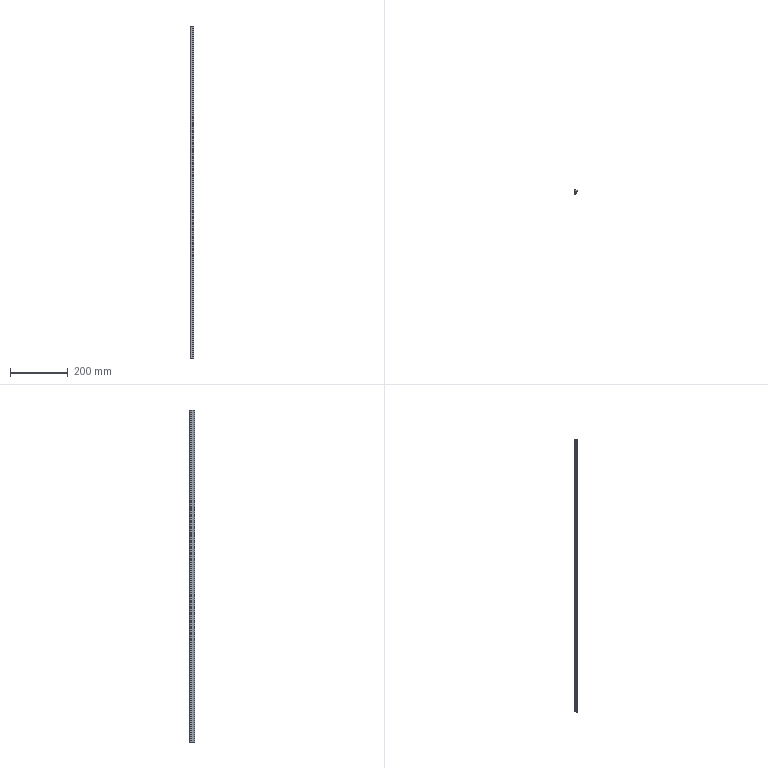Part | SolidWorks | features BaseBody 1, MoveFace 1 | 1 solid | 20 faces | box 10.8 x 17.5 x 1150 mm | volume 90621 mm3 | cylinder 11 | plane 9 | commonest cylinder face diameters 1.6 x2 14 x2 0.4 x1 0.6 x1 0.8 x1 2.6 x1
STEP:
#1=CARTESIAN_POINT('',(-3.236,-11.055,1050.));
#2=VERTEX_POINT('',#1);
#3=CARTESIAN_POINT('',(-4.3,-10.3,1050.));
#4=VERTEX_POINT('',#3);
#5=CARTESIAN_POINT('',(-3.5,-10.3,1050.));
#6=DIRECTION('',(0.,0.,-1.));
#7=DIRECTION('',(1.,0.,0.));
#8=AXIS2_PLACEMENT_3D('',#5,#6,#7);
#9=CIRCLE('',#8,0.8);
#10=EDGE_CURVE('',#2,#4,#9,.T.);
#11=ORIENTED_EDGE('',*,*,#10,.T.);
#12=CARTESIAN_POINT('',(-4.3,-10.3,-100.));
#13=VERTEX_POINT('',#12);
#14=CARTESIAN_POINT('',(-4.3,-10.3,-100.));
#15=DIRECTION('',(0.,0.,-1.));
#16=VECTOR('',#15,1000.);
#17=LINE('',#14,#16);
#18=EDGE_CURVE('',#4,#13,#17,.T.);
#19=ORIENTED_EDGE('',*,*,#18,.T.);
#20=CARTESIAN_POINT('',(-3.236,-11.055,-100.));
#21=VERTEX_POINT('',#20);
#22=CARTESIAN_POINT('',(-3.5,-10.3,-100.));
#23=DIRECTION('',(0.,0.,1.));
#24=DIRECTION('',(-1.,0.,0.));
#25=AXIS2_PLACEMENT_3D('',#22,#23,#24);
#26=CIRCLE('',#25,0.8);
#27=EDGE_CURVE('',#13,#21,#26,.T.);
#28=ORIENTED_EDGE('',*,*,#27,.T.);
#29=CARTESIAN_POINT('',(-3.236,-11.055,-100.));
#30=DIRECTION('',(0.,0.,-1.));
#31=VECTOR('',#30,1000.);
#32=LINE('',#29,#31);
#33=EDGE_CURVE('',#2,#21,#32,.T.);
#34=ORIENTED_EDGE('',*,*,#33,.F.);
#35=EDGE_LOOP('',(#11,#19,#28,#34));
#36=FACE_OUTER_BOUND('',#35,.T.);
#37=CARTESIAN_POINT('',(-3.5,-10.3,-100.));
#38=DIRECTION('',(0.,0.,-1.));
#39=DIRECTION('',(-1.,0.,0.));
#40=AXIS2_PLACEMENT_3D('',#37,#38,#39);
#41=CYLINDRICAL_SURFACE('',#40,0.8);
#42=ADVANCED_FACE('',(#36),#41,.T.);
#43=CARTESIAN_POINT('',(1.184,-6.397,-100.));
#44=VERTEX_POINT('',#43);
#45=CARTESIAN_POINT('',(-5.702,-4.29,-100.));
#46=DIRECTION('',(0.,0.,1.));
#47=DIRECTION('',(-1.,0.,0.));
#48=AXIS2_PLACEMENT_3D('',#45,#46,#47);
#49=CIRCLE('',#48,7.201);
#50=EDGE_CURVE('',#21,#44,#49,.T.);
#51=ORIENTED_EDGE('',*,*,#50,.T.);
#52=CARTESIAN_POINT('',(1.184,-6.397,1050.));
#53=VERTEX_POINT('',#52);
#54=CARTESIAN_POINT('',(1.184,-6.397,-100.));
#55=DIRECTION('',(0.,0.,1.));
#56=VECTOR('',#55,1000.);
#57=LINE('',#54,#56);
#58=EDGE_CURVE('',#44,#53,#57,.T.);
#59=ORIENTED_EDGE('',*,*,#58,.T.);
#60=CARTESIAN_POINT('',(-5.702,-4.29,1050.));
#61=DIRECTION('',(0.,0.,-1.));
#62=DIRECTION('',(1.,0.,0.));
#63=AXIS2_PLACEMENT_3D('',#60,#61,#62);
#64=CIRCLE('',#63,7.201);
#65=EDGE_CURVE('',#53,#2,#64,.T.);
#66=ORIENTED_EDGE('',*,*,#65,.T.);
#67=ORIENTED_EDGE('',*,*,#33,.T.);
#68=EDGE_LOOP('',(#51,#59,#66,#67));
#69=FACE_OUTER_BOUND('',#68,.T.);
#70=CARTESIAN_POINT('',(-5.702,-4.29,-100.));
#71=DIRECTION('',(0.,0.,-1.));
#72=DIRECTION('',(-1.,0.,0.));
#73=AXIS2_PLACEMENT_3D('',#70,#71,#72);
#74=CYLINDRICAL_SURFACE('',#73,7.201);
#75=ADVANCED_FACE('',(#69),#74,.T.);
#76=CARTESIAN_POINT('',(0.9,-6.,-100.));
#77=VERTEX_POINT('',#76);
#78=CARTESIAN_POINT('',(0.9,-6.3,-100.));
#79=DIRECTION('',(0.,0.,1.));
#80=DIRECTION('',(-1.,0.,0.));
#81=AXIS2_PLACEMENT_3D('',#78,#79,#80);
#82=CIRCLE('',#81,0.3);
#83=EDGE_CURVE('',#44,#77,#82,.T.);
#84=ORIENTED_EDGE('',*,*,#83,.T.);
#85=CARTESIAN_POINT('',(0.9,-6.,1050.));
#86=VERTEX_POINT('',#85);
#87=CARTESIAN_POINT('',(0.9,-6.,-100.));
#88=DIRECTION('',(0.,0.,1.));
#89=VECTOR('',#88,1000.);
#90=LINE('',#87,#89);
#91=EDGE_CURVE('',#77,#86,#90,.T.);
#92=ORIENTED_EDGE('',*,*,#91,.T.);
#93=CARTESIAN_POINT('',(0.9,-6.3,1050.));
#94=DIRECTION('',(0.,0.,-1.));
#95=DIRECTION('',(1.,0.,0.));
#96=AXIS2_PLACEMENT_3D('',#93,#94,#95);
#97=CIRCLE('',#96,0.3);
#98=EDGE_CURVE('',#86,#53,#97,.T.);
#99=ORIENTED_EDGE('',*,*,#98,.T.);
#100=ORIENTED_EDGE('',*,*,#58,.F.);
#101=EDGE_LOOP('',(#84,#92,#99,#100));
#102=FACE_OUTER_BOUND('',#101,.T.);
#103=CARTESIAN_POINT('',(0.9,-6.3,-100.));
#104=DIRECTION('',(0.,0.,-1.));
#105=DIRECTION('',(-1.,0.,0.));
#106=AXIS2_PLACEMENT_3D('',#103,#104,#105);
#107=CYLINDRICAL_SURFACE('',#106,0.3);
#108=ADVANCED_FACE('',(#102),#107,.T.);
#109=CARTESIAN_POINT('',(-2.5,-0.5,-100.));
#110=VERTEX_POINT('',#109);
#111=CARTESIAN_POINT('',(-2.5,-6.153,-100.));
#112=VERTEX_POINT('',#111);
#113=CARTESIAN_POINT('',(-2.5,-6.397,-100.));
#114=DIRECTION('',(0.,-1.,0.));
#115=VECTOR('',#114,1000.);
#116=LINE('',#113,#115);
#117=EDGE_CURVE('',#110,#112,#116,.T.);
#118=ORIENTED_EDGE('',*,*,#117,.F.);
#119=CARTESIAN_POINT('',(-4.2,1.695,-100.));
#120=VERTEX_POINT('',#119);
#121=CARTESIAN_POINT('',(-1.701,1.875,-100.));
#122=DIRECTION('',(0.,0.,1.));
#123=DIRECTION('',(-1.,0.,0.));
#124=AXIS2_PLACEMENT_3D('',#121,#122,#123);
#125=CIRCLE('',#124,2.506);
#126=EDGE_CURVE('',#120,#110,#125,.T.);
#127=ORIENTED_EDGE('',*,*,#126,.F.);
#128=CARTESIAN_POINT('',(-4.2,5.1,-100.));
#129=VERTEX_POINT('',#128);
#130=CARTESIAN_POINT('',(-4.2,-6.397,-100.));
#131=DIRECTION('',(0.,-1.,0.));
#132=VECTOR('',#131,1000.);
#133=LINE('',#130,#132);
#134=EDGE_CURVE('',#129,#120,#133,.T.);
#135=ORIENTED_EDGE('',*,*,#134,.F.);
#136=CARTESIAN_POINT('',(-2.892,6.4,-100.));
#137=VERTEX_POINT('',#136);
#138=CARTESIAN_POINT('',(-2.9,5.1,-100.));
#139=DIRECTION('',(0.,0.,1.));
#140=DIRECTION('',(-1.,0.,0.));
#141=AXIS2_PLACEMENT_3D('',#138,#139,#140);
#142=CIRCLE('',#141,1.3);
#143=EDGE_CURVE('',#137,#129,#142,.T.);
#144=ORIENTED_EDGE('',*,*,#143,.F.);
#145=CARTESIAN_POINT('',(0.5,5.5,-100.));
#146=VERTEX_POINT('',#145);
#147=CARTESIAN_POINT('',(-2.934,-0.5999,-100.));
#148=DIRECTION('',(0.,0.,1.));
#149=DIRECTION('',(-1.,0.,0.));
#150=AXIS2_PLACEMENT_3D('',#147,#148,#149);
#151=CIRCLE('',#150,7.);
#152=EDGE_CURVE('',#146,#137,#151,.T.);
#153=ORIENTED_EDGE('',*,*,#152,.F.);
#154=CARTESIAN_POINT('',(5.5,1.7,-100.));
#155=VERTEX_POINT('',#154);
#156=CARTESIAN_POINT('',(5.5,1.7,-100.));
#157=DIRECTION('',(-0.7962,0.6051,0.));
#158=VECTOR('',#157,1000.);
#159=LINE('',#156,#158);
#160=EDGE_CURVE('',#155,#146,#159,.T.);
#161=ORIENTED_EDGE('',*,*,#160,.F.);
#162=CARTESIAN_POINT('',(6.458,-0.2215,-100.));
#163=VERTEX_POINT('',#162);
#164=CARTESIAN_POINT('',(6.458,-0.2215,-100.));
#165=DIRECTION('',(-0.4462,0.8949,0.));
#166=VECTOR('',#165,1000.);
#167=LINE('',#164,#166);
#168=EDGE_CURVE('',#163,#155,#167,.T.);
#169=ORIENTED_EDGE('',*,*,#168,.F.);
#170=CARTESIAN_POINT('',(5.895,-0.7433,-100.));
#171=VERTEX_POINT('',#170);
#172=CARTESIAN_POINT('',(6.1,-0.4,-100.));
#173=DIRECTION('',(0.,0.,1.));
#174=DIRECTION('',(-1.,0.,0.));
#175=AXIS2_PLACEMENT_3D('',#172,#173,#174);
#176=CIRCLE('',#175,0.4);
#177=EDGE_CURVE('',#171,#163,#176,.T.);
#178=ORIENTED_EDGE('',*,*,#177,.F.);
#179=CARTESIAN_POINT('',(3.,0.,-100.));
#180=VERTEX_POINT('',#179);
#181=CARTESIAN_POINT('',(2.746,-6.995,-100.));
#182=DIRECTION('',(0.,0.,-1.));
#183=DIRECTION('',(-1.,0.,0.));
#184=AXIS2_PLACEMENT_3D('',#181,#182,#183);
#185=CIRCLE('',#184,7.);
#186=EDGE_CURVE('',#180,#171,#185,.T.);
#187=ORIENTED_EDGE('',*,*,#186,.F.);
#188=CARTESIAN_POINT('',(0.,0.,-100.));
#189=VERTEX_POINT('',#188);
#190=CARTESIAN_POINT('',(-6.814,0.,-100.));
#191=DIRECTION('',(1.,0.,0.));
#192=VECTOR('',#191,1000.);
#193=LINE('',#190,#192);
#194=EDGE_CURVE('',#189,#180,#193,.T.);
#195=ORIENTED_EDGE('',*,*,#194,.F.);
#196=CARTESIAN_POINT('',(0.,-5.8,-100.));
#197=VERTEX_POINT('',#196);
#198=CARTESIAN_POINT('',(0.,-6.397,-100.));
#199=DIRECTION('',(0.,1.,0.));
#200=VECTOR('',#199,1000.);
#201=LINE('',#198,#200);
#202=EDGE_CURVE('',#197,#189,#201,.T.);
#203=ORIENTED_EDGE('',*,*,#202,.F.);
#204=CARTESIAN_POINT('',(0.2,-6.,-100.));
#205=VERTEX_POINT('',#204);
#206=CARTESIAN_POINT('',(0.2,-5.8,-100.));
#207=DIRECTION('',(0.,0.,1.));
#208=DIRECTION('',(-1.,0.,0.));
#209=AXIS2_PLACEMENT_3D('',#206,#207,#208);
#210=CIRCLE('',#209,0.2);
#211=EDGE_CURVE('',#197,#205,#210,.T.);
#212=ORIENTED_EDGE('',*,*,#211,.T.);
#213=CARTESIAN_POINT('',(-6.814,-6.,-100.));
#214=DIRECTION('',(-1.,0.,0.));
#215=VECTOR('',#214,1000.);
#216=LINE('',#213,#215);
#217=EDGE_CURVE('',#77,#205,#216,.T.);
#218=ORIENTED_EDGE('',*,*,#217,.F.);
#219=ORIENTED_EDGE('',*,*,#83,.F.);
#220=ORIENTED_EDGE('',*,*,#50,.F.);
#221=ORIENTED_EDGE('',*,*,#27,.F.);
#222=CARTESIAN_POINT('',(-3.998,-9.674,-100.));
#223=VERTEX_POINT('',#222);
#224=CARTESIAN_POINT('',(-3.5,-10.3,-100.));
#225=DIRECTION('',(0.,0.,1.));
#226=DIRECTION('',(-1.,0.,0.));
#227=AXIS2_PLACEMENT_3D('',#224,#225,#226);
#228=CIRCLE('',#227,0.8);
#229=EDGE_CURVE('',#223,#13,#228,.T.);
#230=ORIENTED_EDGE('',*,*,#229,.F.);
#231=CARTESIAN_POINT('',(-6.814,-6.397,-100.));
#232=DIRECTION('',(0.,0.,-1.));
#233=DIRECTION('',(-1.,0.,0.));
#234=AXIS2_PLACEMENT_3D('',#231,#232,#233);
#235=CIRCLE('',#234,4.321);
#236=EDGE_CURVE('',#112,#223,#235,.T.);
#237=ORIENTED_EDGE('',*,*,#236,.F.);
#238=EDGE_LOOP('',(#118,#127,#135,#144,#153,#161,#169,#178,#187,#195,#203,#212,#218,#219,#220,#221,#230,#237));
#239=FACE_OUTER_BOUND('',#238,.T.);
#240=CARTESIAN_POINT('',(-6.814,-6.397,-100.));
#241=DIRECTION('',(0.,0.,1.));
#242=DIRECTION('',(1.,0.,0.));
#243=AXIS2_PLACEMENT_3D('',#240,#241,#242);
#244=PLANE('',#243);
#245=ADVANCED_FACE('',(#239),#244,.F.);
#246=ORIENTED_EDGE('',*,*,#18,.F.);
#247=CARTESIAN_POINT('',(-3.998,-9.674,1050.));
#248=VERTEX_POINT('',#247);
#249=CARTESIAN_POINT('',(-3.5,-10.3,1050.));
#250=DIRECTION('',(0.,0.,-1.));
#251=DIRECTION('',(1.,0.,0.));
#252=AXIS2_PLACEMENT_3D('',#249,#250,#251);
#253=CIRCLE('',#252,0.8);
#254=EDGE_CURVE('',#4,#248,#253,.T.);
#255=ORIENTED_EDGE('',*,*,#254,.T.);
#256=CARTESIAN_POINT('',(-3.998,-9.674,-100.));
#257=DIRECTION('',(0.,0.,-1.));
#258=VECTOR('',#257,1000.);
#259=LINE('',#256,#258);
#260=EDGE_CURVE('',#248,#223,#259,.T.);
#261=ORIENTED_EDGE('',*,*,#260,.T.);
#262=ORIENTED_EDGE('',*,*,#229,.T.);
#263=EDGE_LOOP('',(#246,#255,#261,#262));
#264=FACE_OUTER_BOUND('',#263,.T.);
#265=CARTESIAN_POINT('',(-3.5,-10.3,-100.));
#266=DIRECTION('',(0.,0.,-1.));
#267=DIRECTION('',(-1.,0.,0.));
#268=AXIS2_PLACEMENT_3D('',#265,#266,#267);
#269=CYLINDRICAL_SURFACE('',#268,0.8);
#270=ADVANCED_FACE('',(#264),#269,.T.);
#271=CARTESIAN_POINT('',(-4.2,1.695,1050.));
#272=VERTEX_POINT('',#271);
#273=CARTESIAN_POINT('',(-2.5,-0.5,1050.));
#274=VERTEX_POINT('',#273);
#275=CARTESIAN_POINT('',(-1.701,1.875,1050.));
#276=DIRECTION('',(0.,0.,1.));
#277=DIRECTION('',(1.,0.,0.));
#278=AXIS2_PLACEMENT_3D('',#275,#276,#277);
#279=CIRCLE('',#278,2.506);
#280=EDGE_CURVE('',#272,#274,#279,.T.);
#281=ORIENTED_EDGE('',*,*,#280,.T.);
#282=CARTESIAN_POINT('',(-2.5,-6.153,1050.));
#283=VERTEX_POINT('',#282);
#284=CARTESIAN_POINT('',(-2.5,-6.397,1050.));
#285=DIRECTION('',(0.,-1.,0.));
#286=VECTOR('',#285,1000.);
#287=LINE('',#284,#286);
#288=EDGE_CURVE('',#274,#283,#287,.T.);
#289=ORIENTED_EDGE('',*,*,#288,.T.);
#290=CARTESIAN_POINT('',(-6.814,-6.397,1050.));
#291=DIRECTION('',(0.,0.,-1.));
#292=DIRECTION('',(1.,0.,0.));
#293=AXIS2_PLACEMENT_3D('',#290,#291,#292);
#294=CIRCLE('',#293,4.321);
#295=EDGE_CURVE('',#283,#248,#294,.T.);
#296=ORIENTED_EDGE('',*,*,#295,.T.);
#297=ORIENTED_EDGE('',*,*,#254,.F.);
#298=ORIENTED_EDGE('',*,*,#10,.F.);
#299=ORIENTED_EDGE('',*,*,#65,.F.);
#300=ORIENTED_EDGE('',*,*,#98,.F.);
#301=CARTESIAN_POINT('',(0.2,-6.,1050.));
#302=VERTEX_POINT('',#301);
#303=CARTESIAN_POINT('',(-6.814,-6.,1050.));
#304=DIRECTION('',(-1.,0.,0.));
#305=VECTOR('',#304,1000.);
#306=LINE('',#303,#305);
#307=EDGE_CURVE('',#86,#302,#306,.T.);
#308=ORIENTED_EDGE('',*,*,#307,.T.);
#309=CARTESIAN_POINT('',(0.,-5.8,1050.));
#310=VERTEX_POINT('',#309);
#311=CARTESIAN_POINT('',(0.2,-5.8,1050.));
#312=DIRECTION('',(0.,0.,-1.));
#313=DIRECTION('',(1.,0.,0.));
#314=AXIS2_PLACEMENT_3D('',#311,#312,#313);
#315=CIRCLE('',#314,0.2);
#316=EDGE_CURVE('',#302,#310,#315,.T.);
#317=ORIENTED_EDGE('',*,*,#316,.T.);
#318=CARTESIAN_POINT('',(0.,0.,1050.));
#319=VERTEX_POINT('',#318);
#320=CARTESIAN_POINT('',(0.,-6.397,1050.));
#321=DIRECTION('',(0.,1.,0.));
#322=VECTOR('',#321,1000.);
#323=LINE('',#320,#322);
#324=EDGE_CURVE('',#310,#319,#323,.T.);
#325=ORIENTED_EDGE('',*,*,#324,.T.);
#326=CARTESIAN_POINT('',(3.,0.,1050.));
#327=VERTEX_POINT('',#326);
#328=CARTESIAN_POINT('',(-6.814,0.,1050.));
#329=DIRECTION('',(1.,0.,0.));
#330=VECTOR('',#329,1000.);
#331=LINE('',#328,#330);
#332=EDGE_CURVE('',#319,#327,#331,.T.);
#333=ORIENTED_EDGE('',*,*,#332,.T.);
#334=CARTESIAN_POINT('',(5.895,-0.7433,1050.));
#335=VERTEX_POINT('',#334);
#336=CARTESIAN_POINT('',(2.746,-6.995,1050.));
#337=DIRECTION('',(0.,0.,-1.));
#338=DIRECTION('',(1.,0.,0.));
#339=AXIS2_PLACEMENT_3D('',#336,#337,#338);
#340=CIRCLE('',#339,7.);
#341=EDGE_CURVE('',#327,#335,#340,.T.);
#342=ORIENTED_EDGE('',*,*,#341,.T.);
#343=CARTESIAN_POINT('',(6.458,-0.2215,1050.));
#344=VERTEX_POINT('',#343);
#345=CARTESIAN_POINT('',(6.1,-0.4,1050.));
#346=DIRECTION('',(0.,0.,-1.));
#347=DIRECTION('',(1.,0.,0.));
#348=AXIS2_PLACEMENT_3D('',#345,#346,#347);
#349=CIRCLE('',#348,0.4);
#350=EDGE_CURVE('',#344,#335,#349,.T.);
#351=ORIENTED_EDGE('',*,*,#350,.F.);
#352=CARTESIAN_POINT('',(5.5,1.7,1050.));
#353=VERTEX_POINT('',#352);
#354=CARTESIAN_POINT('',(6.282,0.1323,1050.));
#355=DIRECTION('',(-0.4462,0.8949,0.));
#356=VECTOR('',#355,1000.);
#357=LINE('',#354,#356);
#358=EDGE_CURVE('',#344,#353,#357,.T.);
#359=ORIENTED_EDGE('',*,*,#358,.T.);
#360=CARTESIAN_POINT('',(0.5,5.5,1050.));
#361=VERTEX_POINT('',#360);
#362=CARTESIAN_POINT('',(1.595,4.668,1050.));
#363=DIRECTION('',(-0.7962,0.6051,0.));
#364=VECTOR('',#363,1000.);
#365=LINE('',#362,#364);
#366=EDGE_CURVE('',#353,#361,#365,.T.);
#367=ORIENTED_EDGE('',*,*,#366,.T.);
#368=CARTESIAN_POINT('',(-2.892,6.4,1050.));
#369=VERTEX_POINT('',#368);
#370=CARTESIAN_POINT('',(-2.934,-0.5999,1050.));
#371=DIRECTION('',(0.,0.,1.));
#372=DIRECTION('',(1.,0.,0.));
#373=AXIS2_PLACEMENT_3D('',#370,#371,#372);
#374=CIRCLE('',#373,7.);
#375=EDGE_CURVE('',#361,#369,#374,.T.);
#376=ORIENTED_EDGE('',*,*,#375,.T.);
#377=CARTESIAN_POINT('',(-4.2,5.1,1050.));
#378=VERTEX_POINT('',#377);
#379=CARTESIAN_POINT('',(-2.9,5.1,1050.));
#380=DIRECTION('',(0.,0.,1.));
#381=DIRECTION('',(1.,0.,0.));
#382=AXIS2_PLACEMENT_3D('',#379,#380,#381);
#383=CIRCLE('',#382,1.3);
#384=EDGE_CURVE('',#369,#378,#383,.T.);
#385=ORIENTED_EDGE('',*,*,#384,.T.);
#386=CARTESIAN_POINT('',(-4.2,-6.397,1050.));
#387=DIRECTION('',(0.,-1.,0.));
#388=VECTOR('',#387,1000.);
#389=LINE('',#386,#388);
#390=EDGE_CURVE('',#378,#272,#389,.T.);
#391=ORIENTED_EDGE('',*,*,#390,.T.);
#392=EDGE_LOOP('',(#281,#289,#296,#297,#298,#299,#300,#308,#317,#325,#333,#342,#351,#359,#367,#376,#385,#391));
#393=FACE_OUTER_BOUND('',#392,.T.);
#394=CARTESIAN_POINT('',(-6.814,-6.397,1050.));
#395=DIRECTION('',(0.,0.,1.));
#396=DIRECTION('',(1.,0.,0.));
#397=AXIS2_PLACEMENT_3D('',#394,#395,#396);
#398=PLANE('',#397);
#399=ADVANCED_FACE('',(#393),#398,.T.);
#400=ORIENTED_EDGE('',*,*,#217,.T.);
#401=CARTESIAN_POINT('',(0.2,-6.,-100.));
#402=DIRECTION('',(0.,0.,1.));
#403=VECTOR('',#402,1000.);
#404=LINE('',#401,#403);
#405=EDGE_CURVE('',#205,#302,#404,.T.);
#406=ORIENTED_EDGE('',*,*,#405,.T.);
#407=ORIENTED_EDGE('',*,*,#307,.F.);
#408=ORIENTED_EDGE('',*,*,#91,.F.);
#409=EDGE_LOOP('',(#400,#406,#407,#408));
#410=FACE_OUTER_BOUND('',#409,.T.);
#411=CARTESIAN_POINT('',(0.9,-6.,-100.));
#412=DIRECTION('',(0.,1.,0.));
#413=DIRECTION('',(0.,0.,1.));
#414=AXIS2_PLACEMENT_3D('',#411,#412,#413);
#415=PLANE('',#414);
#416=ADVANCED_FACE('',(#410),#415,.T.);
#417=CARTESIAN_POINT('',(-2.5,-6.153,-100.));
#418=DIRECTION('',(0.,0.,1.));
#419=VECTOR('',#418,1000.);
#420=LINE('',#417,#419);
#421=EDGE_CURVE('',#112,#283,#420,.T.);
#422=ORIENTED_EDGE('',*,*,#421,.F.);
#423=ORIENTED_EDGE('',*,*,#236,.T.);
#424=ORIENTED_EDGE('',*,*,#260,.F.);
#425=ORIENTED_EDGE('',*,*,#295,.F.);
#426=EDGE_LOOP('',(#422,#423,#424,#425));
#427=FACE_OUTER_BOUND('',#426,.T.);
#428=CARTESIAN_POINT('',(-6.814,-6.397,-100.));
#429=DIRECTION('',(0.,0.,-1.));
#430=DIRECTION('',(-1.,0.,0.));
#431=AXIS2_PLACEMENT_3D('',#428,#429,#430);
#432=CYLINDRICAL_SURFACE('',#431,4.321);
#433=ADVANCED_FACE('',(#427),#432,.F.);
#434=ORIENTED_EDGE('',*,*,#117,.T.);
#435=ORIENTED_EDGE('',*,*,#421,.T.);
#436=ORIENTED_EDGE('',*,*,#288,.F.);
#437=CARTESIAN_POINT('',(-2.5,-0.5,-100.));
#438=DIRECTION('',(0.,0.,-1.));
#439=VECTOR('',#438,1000.);
#440=LINE('',#437,#439);
#441=EDGE_CURVE('',#274,#110,#440,.T.);
#442=ORIENTED_EDGE('',*,*,#441,.T.);
#443=EDGE_LOOP('',(#434,#435,#436,#442));
#444=FACE_OUTER_BOUND('',#443,.T.);
#445=CARTESIAN_POINT('',(-2.5,-0.5,-100.));
#446=DIRECTION('',(-1.,0.,0.));
#447=DIRECTION('',(0.,0.,1.));
#448=AXIS2_PLACEMENT_3D('',#445,#446,#447);
#449=PLANE('',#448);
#450=ADVANCED_FACE('',(#444),#449,.T.);
#451=ORIENTED_EDGE('',*,*,#126,.T.);
#452=ORIENTED_EDGE('',*,*,#441,.F.);
#453=ORIENTED_EDGE('',*,*,#280,.F.);
#454=CARTESIAN_POINT('',(-4.2,1.695,-100.));
#455=DIRECTION('',(0.,0.,-1.));
#456=VECTOR('',#455,1000.);
#457=LINE('',#454,#456);
#458=EDGE_CURVE('',#272,#120,#457,.T.);
#459=ORIENTED_EDGE('',*,*,#458,.T.);
#460=EDGE_LOOP('',(#451,#452,#453,#459));
#461=FACE_OUTER_BOUND('',#460,.T.);
#462=CARTESIAN_POINT('',(-1.701,1.875,-100.));
#463=DIRECTION('',(0.,0.,-1.));
#464=DIRECTION('',(-1.,0.,0.));
#465=AXIS2_PLACEMENT_3D('',#462,#463,#464);
#466=CYLINDRICAL_SURFACE('',#465,2.506);
#467=ADVANCED_FACE('',(#461),#466,.T.);
#468=ORIENTED_EDGE('',*,*,#134,.T.);
#469=ORIENTED_EDGE('',*,*,#458,.F.);
#470=ORIENTED_EDGE('',*,*,#390,.F.);
#471=CARTESIAN_POINT('',(-4.2,5.1,-100.));
#472=DIRECTION('',(0.,0.,-1.));
#473=VECTOR('',#472,1000.);
#474=LINE('',#471,#473);
#475=EDGE_CURVE('',#378,#129,#474,.T.);
#476=ORIENTED_EDGE('',*,*,#475,.T.);
#477=EDGE_LOOP('',(#468,#469,#470,#476));
#478=FACE_OUTER_BOUND('',#477,.T.);
#479=CARTESIAN_POINT('',(-4.2,5.1,-100.));
#480=DIRECTION('',(-1.,0.,0.));
#481=DIRECTION('',(0.,0.,1.));
#482=AXIS2_PLACEMENT_3D('',#479,#480,#481);
#483=PLANE('',#482);
#484=ADVANCED_FACE('',(#478),#483,.T.);
#485=ORIENTED_EDGE('',*,*,#143,.T.);
#486=ORIENTED_EDGE('',*,*,#475,.F.);
#487=ORIENTED_EDGE('',*,*,#384,.F.);
#488=CARTESIAN_POINT('',(-2.892,6.4,-100.));
#489=DIRECTION('',(0.,0.,-1.));
#490=VECTOR('',#489,1000.);
#491=LINE('',#488,#490);
#492=EDGE_CURVE('',#369,#137,#491,.T.);
#493=ORIENTED_EDGE('',*,*,#492,.T.);
#494=EDGE_LOOP('',(#485,#486,#487,#493));
#495=FACE_OUTER_BOUND('',#494,.T.);
#496=CARTESIAN_POINT('',(-2.9,5.1,-100.));
#497=DIRECTION('',(0.,0.,-1.));
#498=DIRECTION('',(-1.,0.,0.));
#499=AXIS2_PLACEMENT_3D('',#496,#497,#498);
#500=CYLINDRICAL_SURFACE('',#499,1.3);
#501=ADVANCED_FACE('',(#495),#500,.T.);
#502=ORIENTED_EDGE('',*,*,#152,.T.);
#503=ORIENTED_EDGE('',*,*,#492,.F.);
#504=ORIENTED_EDGE('',*,*,#375,.F.);
#505=CARTESIAN_POINT('',(0.5,5.5,-100.));
#506=DIRECTION('',(0.,0.,-1.));
#507=VECTOR('',#506,1000.);
#508=LINE('',#505,#507);
#509=EDGE_CURVE('',#361,#146,#508,.T.);
#510=ORIENTED_EDGE('',*,*,#509,.T.);
#511=EDGE_LOOP('',(#502,#503,#504,#510));
#512=FACE_OUTER_BOUND('',#511,.T.);
#513=CARTESIAN_POINT('',(-2.934,-0.5999,-100.));
#514=DIRECTION('',(0.,0.,-1.));
#515=DIRECTION('',(-1.,0.,0.));
#516=AXIS2_PLACEMENT_3D('',#513,#514,#515);
#517=CYLINDRICAL_SURFACE('',#516,7.);
#518=ADVANCED_FACE('',(#512),#517,.T.);
#519=ORIENTED_EDGE('',*,*,#160,.T.);
#520=ORIENTED_EDGE('',*,*,#509,.F.);
#521=ORIENTED_EDGE('',*,*,#366,.F.);
#522=CARTESIAN_POINT('',(5.5,1.7,-100.));
#523=DIRECTION('',(0.,0.,-1.));
#524=VECTOR('',#523,1000.);
#525=LINE('',#522,#524);
#526=EDGE_CURVE('',#353,#155,#525,.T.);
#527=ORIENTED_EDGE('',*,*,#526,.T.);
#528=EDGE_LOOP('',(#519,#520,#521,#527));
#529=FACE_OUTER_BOUND('',#528,.T.);
#530=CARTESIAN_POINT('',(5.5,1.7,-100.));
#531=DIRECTION('',(0.6051,0.7962,0.));
#532=DIRECTION('',(-0.7962,0.6051,0.));
#533=AXIS2_PLACEMENT_3D('',#530,#531,#532);
#534=PLANE('',#533);
#535=ADVANCED_FACE('',(#529),#534,.T.);
#536=ORIENTED_EDGE('',*,*,#168,.T.);
#537=ORIENTED_EDGE('',*,*,#526,.F.);
#538=ORIENTED_EDGE('',*,*,#358,.F.);
#539=CARTESIAN_POINT('',(6.458,-0.2215,-100.));
#540=DIRECTION('',(0.,0.,-1.));
#541=VECTOR('',#540,1000.);
#542=LINE('',#539,#541);
#543=EDGE_CURVE('',#344,#163,#542,.T.);
#544=ORIENTED_EDGE('',*,*,#543,.T.);
#545=EDGE_LOOP('',(#536,#537,#538,#544));
#546=FACE_OUTER_BOUND('',#545,.T.);
#547=CARTESIAN_POINT('',(6.458,-0.2215,-100.));
#548=DIRECTION('',(0.8949,0.4462,0.));
#549=DIRECTION('',(-0.4462,0.8949,0.));
#550=AXIS2_PLACEMENT_3D('',#547,#548,#549);
#551=PLANE('',#550);
#552=ADVANCED_FACE('',(#546),#551,.T.);
#553=CARTESIAN_POINT('',(3.,0.,-100.));
#554=DIRECTION('',(0.,0.,1.));
#555=VECTOR('',#554,1000.);
#556=LINE('',#553,#555);
#557=EDGE_CURVE('',#180,#327,#556,.T.);
#558=ORIENTED_EDGE('',*,*,#557,.F.);
#559=ORIENTED_EDGE('',*,*,#186,.T.);
#560=CARTESIAN_POINT('',(5.895,-0.7433,-100.));
#561=DIRECTION('',(0.,0.,-1.));
#562=VECTOR('',#561,1000.);
#563=LINE('',#560,#562);
#564=EDGE_CURVE('',#335,#171,#563,.T.);
#565=ORIENTED_EDGE('',*,*,#564,.F.);
#566=ORIENTED_EDGE('',*,*,#341,.F.);
#567=EDGE_LOOP('',(#558,#559,#565,#566));
#568=FACE_OUTER_BOUND('',#567,.T.);
#569=CARTESIAN_POINT('',(2.746,-6.995,-100.));
#570=DIRECTION('',(0.,0.,-1.));
#571=DIRECTION('',(-1.,0.,0.));
#572=AXIS2_PLACEMENT_3D('',#569,#570,#571);
#573=CYLINDRICAL_SURFACE('',#572,7.);
#574=ADVANCED_FACE('',(#568),#573,.F.);
#575=ORIENTED_EDGE('',*,*,#194,.T.);
#576=ORIENTED_EDGE('',*,*,#557,.T.);
#577=ORIENTED_EDGE('',*,*,#332,.F.);
#578=CARTESIAN_POINT('',(0.,0.,-100.));
#579=DIRECTION('',(0.,0.,-1.));
#580=VECTOR('',#579,1000.);
#581=LINE('',#578,#580);
#582=EDGE_CURVE('',#319,#189,#581,.T.);
#583=ORIENTED_EDGE('',*,*,#582,.T.);
#584=EDGE_LOOP('',(#575,#576,#577,#583));
#585=FACE_OUTER_BOUND('',#584,.T.);
#586=CARTESIAN_POINT('',(0.,0.,-100.));
#587=DIRECTION('',(0.,-1.,0.));
#588=DIRECTION('',(0.,0.,-1.));
#589=AXIS2_PLACEMENT_3D('',#586,#587,#588);
#590=PLANE('',#589);
#591=ADVANCED_FACE('',(#585),#590,.T.);
#592=ORIENTED_EDGE('',*,*,#202,.T.);
#593=ORIENTED_EDGE('',*,*,#582,.F.);
#594=ORIENTED_EDGE('',*,*,#324,.F.);
#595=CARTESIAN_POINT('',(0.,-5.8,-100.));
#596=DIRECTION('',(0.,0.,-1.));
#597=VECTOR('',#596,1000.);
#598=LINE('',#595,#597);
#599=EDGE_CURVE('',#310,#197,#598,.T.);
#600=ORIENTED_EDGE('',*,*,#599,.T.);
#601=EDGE_LOOP('',(#592,#593,#594,#600));
#602=FACE_OUTER_BOUND('',#601,.T.);
#603=CARTESIAN_POINT('',(0.,-5.8,-100.));
#604=DIRECTION('',(1.,0.,0.));
#605=DIRECTION('',(0.,0.,-1.));
#606=AXIS2_PLACEMENT_3D('',#603,#604,#605);
#607=PLANE('',#606);
#608=ADVANCED_FACE('',(#602),#607,.T.);
#609=ORIENTED_EDGE('',*,*,#405,.F.);
#610=ORIENTED_EDGE('',*,*,#211,.F.);
#611=ORIENTED_EDGE('',*,*,#599,.F.);
#612=ORIENTED_EDGE('',*,*,#316,.F.);
#613=EDGE_LOOP('',(#609,#610,#611,#612));
#614=FACE_OUTER_BOUND('',#613,.T.);
#615=CARTESIAN_POINT('',(0.2,-5.8,-100.));
#616=DIRECTION('',(0.,0.,-1.));
#617=DIRECTION('',(-1.,0.,0.));
#618=AXIS2_PLACEMENT_3D('',#615,#616,#617);
#619=CYLINDRICAL_SURFACE('',#618,0.2);
#620=ADVANCED_FACE('',(#614),#619,.F.);
#621=ORIENTED_EDGE('',*,*,#177,.T.);
#622=ORIENTED_EDGE('',*,*,#543,.F.);
#623=ORIENTED_EDGE('',*,*,#350,.T.);
#624=ORIENTED_EDGE('',*,*,#564,.T.);
#625=EDGE_LOOP('',(#621,#622,#623,#624));
#626=FACE_OUTER_BOUND('',#625,.T.);
#627=CARTESIAN_POINT('',(6.1,-0.4,-100.));
#628=DIRECTION('',(0.,0.,-1.));
#629=DIRECTION('',(-1.,0.,0.));
#630=AXIS2_PLACEMENT_3D('',#627,#628,#629);
#631=CYLINDRICAL_SURFACE('',#630,0.4);
#632=ADVANCED_FACE('',(#626),#631,.T.);
#633=CLOSED_SHELL('',(#42,#75,#108,#245,#270,#399,#416,#433,#450,#467,#484,#501,#518,#535,#552,#574,#591,#608,#620,#632));
#634=MANIFOLD_SOLID_BREP('',#633);
#635=CARTESIAN_POINT('',(0.,0.,0.));
#636=DIRECTION('',(0.,0.,1.));
#637=DIRECTION('',(1.,0.,0.));
#638=AXIS2_PLACEMENT_3D('',#635,#636,#637);
#639=(LENGTH_UNIT()NAMED_UNIT(*)SI_UNIT(.MILLI.,.METRE.));
#640=UNCERTAINTY_MEASURE_WITH_UNIT(LENGTH_MEASURE(0.00001),#639,'','');
#641=(NAMED_UNIT(*)PLANE_ANGLE_UNIT()SI_UNIT($,.RADIAN.));
#642=(NAMED_UNIT(*)SI_UNIT($,.STERADIAN.)SOLID_ANGLE_UNIT());
#643=(GEOMETRIC_REPRESENTATION_CONTEXT(3)GLOBAL_UNCERTAINTY_ASSIGNED_CONTEXT((#640))GLOBAL_UNIT_ASSIGNED_CONTEXT((#639,#641,#642))REPRESENTATION_CONTEXT('',''));
#644=ADVANCED_BREP_SHAPE_REPRESENTATION('',(#634,#638),#643);